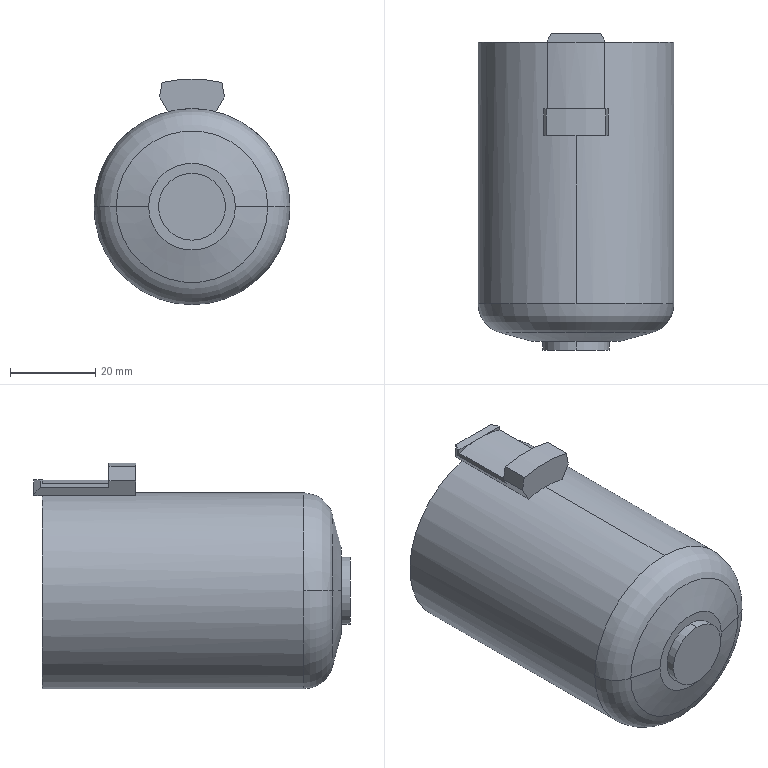Part | STEP file | _AL30-A_BOWL | 1 solid | 29 faces | box 46 x 74.3 x 53 mm | volume 115027 mm3 | plane 17 | cylinder 8 | torus 2 | cone 2 | commonest cylinder face diameters 46 x4 15.7 x2 52 x1 60 x1
STEP:
#1=CARTESIAN_POINT('',(23.,-93.199,0.));
#2=VERTEX_POINT('',#1);
#3=CARTESIAN_POINT('',(0.,-93.199,-23.));
#4=VERTEX_POINT('',#3);
#5=CARTESIAN_POINT('',(0.,-93.199,0.));
#6=DIRECTION('',(0.,1.,0.));
#7=DIRECTION('',(0.,0.,1.));
#8=AXIS2_PLACEMENT_3D('',#5,#6,#7);
#9=CIRCLE('',#8,23.);
#10=EDGE_CURVE('',#2,#4,#9,.T.);
#11=ORIENTED_EDGE('',*,*,#10,.T.);
#12=CARTESIAN_POINT('',(0.,-31.8,-23.));
#13=VERTEX_POINT('',#12);
#14=CARTESIAN_POINT('',(0.,-104.1,-23.));
#15=DIRECTION('',(0.,1.,0.));
#16=VECTOR('',#15,1000.);
#17=LINE('',#14,#16);
#18=EDGE_CURVE('',#4,#13,#17,.T.);
#19=ORIENTED_EDGE('',*,*,#18,.T.);
#20=CARTESIAN_POINT('',(5.604,-31.8,22.307));
#21=VERTEX_POINT('',#20);
#22=CARTESIAN_POINT('',(0.,-31.8,0.));
#23=DIRECTION('',(0.,-1.,0.));
#24=DIRECTION('',(0.,0.,1.));
#25=AXIS2_PLACEMENT_3D('',#22,#23,#24);
#26=CIRCLE('',#25,23.);
#27=EDGE_CURVE('',#13,#21,#26,.T.);
#28=ORIENTED_EDGE('',*,*,#27,.T.);
#29=CARTESIAN_POINT('',(5.604,-53.76,22.307));
#30=VERTEX_POINT('',#29);
#31=CARTESIAN_POINT('',(5.604,-104.1,22.307));
#32=DIRECTION('',(0.,-1.,0.));
#33=VECTOR('',#32,1000.);
#34=LINE('',#31,#33);
#35=EDGE_CURVE('',#21,#30,#34,.T.);
#36=ORIENTED_EDGE('',*,*,#35,.T.);
#37=CARTESIAN_POINT('',(0.,-53.76,23.));
#38=VERTEX_POINT('',#37);
#39=CARTESIAN_POINT('',(0.,-53.76,0.));
#40=DIRECTION('',(0.,-1.,0.));
#41=DIRECTION('',(0.,0.,1.));
#42=AXIS2_PLACEMENT_3D('',#39,#40,#41);
#43=CIRCLE('',#42,23.);
#44=EDGE_CURVE('',#30,#38,#43,.T.);
#45=ORIENTED_EDGE('',*,*,#44,.T.);
#46=CARTESIAN_POINT('',(0.,-93.199,23.));
#47=VERTEX_POINT('',#46);
#48=CARTESIAN_POINT('',(0.,-104.1,23.));
#49=DIRECTION('',(0.,1.,0.));
#50=VECTOR('',#49,1000.);
#51=LINE('',#48,#50);
#52=EDGE_CURVE('',#47,#38,#51,.T.);
#53=ORIENTED_EDGE('',*,*,#52,.F.);
#54=CARTESIAN_POINT('',(0.,-93.199,0.));
#55=DIRECTION('',(0.,1.,0.));
#56=DIRECTION('',(0.,0.,1.));
#57=AXIS2_PLACEMENT_3D('',#54,#55,#56);
#58=CIRCLE('',#57,23.);
#59=EDGE_CURVE('',#47,#2,#58,.T.);
#60=ORIENTED_EDGE('',*,*,#59,.T.);
#61=EDGE_LOOP('',(#11,#19,#28,#36,#45,#53,#60));
#62=FACE_OUTER_BOUND('',#61,.T.);
#63=CARTESIAN_POINT('',(0.,-104.1,0.));
#64=DIRECTION('',(0.,1.,0.));
#65=DIRECTION('',(0.,0.,1.));
#66=AXIS2_PLACEMENT_3D('',#63,#64,#65);
#67=CYLINDRICAL_SURFACE('',#66,23.);
#68=ADVANCED_FACE('',(#62),#67,.T.);
#69=CARTESIAN_POINT('',(-23.,-93.199,0.));
#70=VERTEX_POINT('',#69);
#71=CARTESIAN_POINT('',(0.,-93.199,0.));
#72=DIRECTION('',(0.,1.,0.));
#73=DIRECTION('',(0.,0.,1.));
#74=AXIS2_PLACEMENT_3D('',#71,#72,#73);
#75=CIRCLE('',#74,23.);
#76=EDGE_CURVE('',#70,#47,#75,.T.);
#77=ORIENTED_EDGE('',*,*,#76,.F.);
#78=CARTESIAN_POINT('',(-17.812,-99.96,0.));
#79=VERTEX_POINT('',#78);
#80=CARTESIAN_POINT('',(-16.,-93.199,0.));
#81=DIRECTION('',(0.,0.,1.));
#82=DIRECTION('',(1.,0.,0.));
#83=AXIS2_PLACEMENT_3D('',#80,#81,#82);
#84=CIRCLE('',#83,7.);
#85=EDGE_CURVE('',#70,#79,#84,.T.);
#86=ORIENTED_EDGE('',*,*,#85,.T.);
#87=CARTESIAN_POINT('',(17.812,-99.96,0.));
#88=VERTEX_POINT('',#87);
#89=CARTESIAN_POINT('',(0.,-99.96,0.));
#90=DIRECTION('',(0.,1.,0.));
#91=DIRECTION('',(0.,0.,-1.));
#92=AXIS2_PLACEMENT_3D('',#89,#90,#91);
#93=CIRCLE('',#92,17.812);
#94=EDGE_CURVE('',#79,#88,#93,.T.);
#95=ORIENTED_EDGE('',*,*,#94,.T.);
#96=CARTESIAN_POINT('',(16.,-93.199,0.));
#97=DIRECTION('',(0.,0.,-1.));
#98=DIRECTION('',(-1.,0.,0.));
#99=AXIS2_PLACEMENT_3D('',#96,#97,#98);
#100=CIRCLE('',#99,7.);
#101=EDGE_CURVE('',#2,#88,#100,.T.);
#102=ORIENTED_EDGE('',*,*,#101,.F.);
#103=ORIENTED_EDGE('',*,*,#59,.F.);
#104=EDGE_LOOP('',(#77,#86,#95,#102,#103));
#105=FACE_OUTER_BOUND('',#104,.T.);
#106=CARTESIAN_POINT('',(0.,-93.199,0.));
#107=DIRECTION('',(0.,-1.,0.));
#108=DIRECTION('',(1.,0.,0.));
#109=AXIS2_PLACEMENT_3D('',#106,#107,#108);
#110=TOROIDAL_SURFACE('',#109,16.,7.);
#111=ADVANCED_FACE('',(#105),#110,.T.);
#112=CARTESIAN_POINT('',(0.,-31.8,23.));
#113=VERTEX_POINT('',#112);
#114=CARTESIAN_POINT('',(0.,-31.8,0.));
#115=DIRECTION('',(0.,-1.,0.));
#116=DIRECTION('',(0.,0.,1.));
#117=AXIS2_PLACEMENT_3D('',#114,#115,#116);
#118=CIRCLE('',#117,23.);
#119=EDGE_CURVE('',#21,#113,#118,.T.);
#120=ORIENTED_EDGE('',*,*,#119,.T.);
#121=CARTESIAN_POINT('',(0.,-29.8,23.));
#122=VERTEX_POINT('',#121);
#123=CARTESIAN_POINT('',(0.,-29.8,23.));
#124=DIRECTION('',(0.,1.,0.));
#125=VECTOR('',#124,1000.);
#126=LINE('',#123,#125);
#127=EDGE_CURVE('',#113,#122,#126,.T.);
#128=ORIENTED_EDGE('',*,*,#127,.T.);
#129=CARTESIAN_POINT('',(5.604,-29.8,22.307));
#130=VERTEX_POINT('',#129);
#131=CARTESIAN_POINT('',(0.,-29.8,0.));
#132=DIRECTION('',(0.,-1.,0.));
#133=DIRECTION('',(0.,0.,1.));
#134=AXIS2_PLACEMENT_3D('',#131,#132,#133);
#135=CIRCLE('',#134,23.);
#136=EDGE_CURVE('',#130,#122,#135,.T.);
#137=ORIENTED_EDGE('',*,*,#136,.F.);
#138=CARTESIAN_POINT('',(5.604,-47.45,22.307));
#139=DIRECTION('',(0.,1.,0.));
#140=VECTOR('',#139,1000.);
#141=LINE('',#138,#140);
#142=EDGE_CURVE('',#21,#130,#141,.T.);
#143=ORIENTED_EDGE('',*,*,#142,.F.);
#144=EDGE_LOOP('',(#120,#128,#137,#143));
#145=FACE_OUTER_BOUND('',#144,.T.);
#146=CARTESIAN_POINT('',(0.,-29.8,0.));
#147=DIRECTION('',(0.,1.,0.));
#148=DIRECTION('',(0.,0.,1.));
#149=AXIS2_PLACEMENT_3D('',#146,#147,#148);
#150=CYLINDRICAL_SURFACE('',#149,23.);
#151=ADVANCED_FACE('',(#145),#150,.F.);
#152=CARTESIAN_POINT('',(-10.2,-102.,0.));
#153=VERTEX_POINT('',#152);
#154=CARTESIAN_POINT('',(10.2,-102.,0.));
#155=VERTEX_POINT('',#154);
#156=CARTESIAN_POINT('',(0.,-102.,0.));
#157=DIRECTION('',(0.,1.,0.));
#158=DIRECTION('',(-1.,0.,0.));
#159=AXIS2_PLACEMENT_3D('',#156,#157,#158);
#160=CIRCLE('',#159,10.2);
#161=EDGE_CURVE('',#153,#155,#160,.T.);
#162=ORIENTED_EDGE('',*,*,#161,.T.);
#163=CARTESIAN_POINT('',(17.812,-99.96,0.));
#164=DIRECTION('',(0.9659,0.2588,0.));
#165=VECTOR('',#164,1000.);
#166=LINE('',#163,#165);
#167=EDGE_CURVE('',#155,#88,#166,.T.);
#168=ORIENTED_EDGE('',*,*,#167,.T.);
#169=ORIENTED_EDGE('',*,*,#94,.F.);
#170=CARTESIAN_POINT('',(-17.812,-99.96,0.));
#171=DIRECTION('',(-0.9659,0.2588,0.));
#172=VECTOR('',#171,1000.);
#173=LINE('',#170,#172);
#174=EDGE_CURVE('',#153,#79,#173,.T.);
#175=ORIENTED_EDGE('',*,*,#174,.F.);
#176=EDGE_LOOP('',(#162,#168,#169,#175));
#177=FACE_OUTER_BOUND('',#176,.T.);
#178=CARTESIAN_POINT('',(0.,-99.96,0.));
#179=DIRECTION('',(0.,1.,0.));
#180=DIRECTION('',(-1.,0.,0.));
#181=AXIS2_PLACEMENT_3D('',#178,#179,#180);
#182=CONICAL_SURFACE('',#181,17.812,1.309);
#183=ADVANCED_FACE('',(#177),#182,.T.);
#184=CARTESIAN_POINT('',(0.,-104.1,7.85));
#185=VERTEX_POINT('',#184);
#186=CARTESIAN_POINT('',(0.,-104.1,-7.85));
#187=VERTEX_POINT('',#186);
#188=CARTESIAN_POINT('',(0.,-104.1,0.));
#189=DIRECTION('',(0.,1.,0.));
#190=DIRECTION('',(0.,0.,1.));
#191=AXIS2_PLACEMENT_3D('',#188,#189,#190);
#192=CIRCLE('',#191,7.85);
#193=EDGE_CURVE('',#185,#187,#192,.T.);
#194=ORIENTED_EDGE('',*,*,#193,.T.);
#195=CARTESIAN_POINT('',(0.,-102.,-7.85));
#196=VERTEX_POINT('',#195);
#197=CARTESIAN_POINT('',(0.,-104.1,-7.85));
#198=DIRECTION('',(0.,1.,0.));
#199=VECTOR('',#198,1000.);
#200=LINE('',#197,#199);
#201=EDGE_CURVE('',#187,#196,#200,.T.);
#202=ORIENTED_EDGE('',*,*,#201,.T.);
#203=CARTESIAN_POINT('',(0.,-102.,7.85));
#204=VERTEX_POINT('',#203);
#205=CARTESIAN_POINT('',(0.,-102.,0.));
#206=DIRECTION('',(0.,-1.,0.));
#207=DIRECTION('',(0.,0.,1.));
#208=AXIS2_PLACEMENT_3D('',#205,#206,#207);
#209=CIRCLE('',#208,7.85);
#210=EDGE_CURVE('',#196,#204,#209,.T.);
#211=ORIENTED_EDGE('',*,*,#210,.T.);
#212=CARTESIAN_POINT('',(0.,-104.1,7.85));
#213=DIRECTION('',(0.,1.,0.));
#214=VECTOR('',#213,1000.);
#215=LINE('',#212,#214);
#216=EDGE_CURVE('',#185,#204,#215,.T.);
#217=ORIENTED_EDGE('',*,*,#216,.F.);
#218=EDGE_LOOP('',(#194,#202,#211,#217));
#219=FACE_OUTER_BOUND('',#218,.T.);
#220=CARTESIAN_POINT('',(0.,-104.1,0.));
#221=DIRECTION('',(0.,1.,0.));
#222=DIRECTION('',(0.,0.,1.));
#223=AXIS2_PLACEMENT_3D('',#220,#221,#222);
#224=CYLINDRICAL_SURFACE('',#223,7.85);
#225=ADVANCED_FACE('',(#219),#224,.T.);
#226=ORIENTED_EDGE('',*,*,#18,.F.);
#227=CARTESIAN_POINT('',(0.,-93.199,0.));
#228=DIRECTION('',(0.,1.,0.));
#229=DIRECTION('',(0.,0.,1.));
#230=AXIS2_PLACEMENT_3D('',#227,#228,#229);
#231=CIRCLE('',#230,23.);
#232=EDGE_CURVE('',#4,#70,#231,.T.);
#233=ORIENTED_EDGE('',*,*,#232,.T.);
#234=ORIENTED_EDGE('',*,*,#76,.T.);
#235=ORIENTED_EDGE('',*,*,#52,.T.);
#236=CARTESIAN_POINT('',(-5.604,-53.76,22.307));
#237=VERTEX_POINT('',#236);
#238=CARTESIAN_POINT('',(0.,-53.76,0.));
#239=DIRECTION('',(0.,-1.,0.));
#240=DIRECTION('',(0.,0.,1.));
#241=AXIS2_PLACEMENT_3D('',#238,#239,#240);
#242=CIRCLE('',#241,23.);
#243=EDGE_CURVE('',#38,#237,#242,.T.);
#244=ORIENTED_EDGE('',*,*,#243,.T.);
#245=CARTESIAN_POINT('',(-5.604,-31.8,22.307));
#246=VERTEX_POINT('',#245);
#247=CARTESIAN_POINT('',(-5.604,-104.1,22.307));
#248=DIRECTION('',(0.,1.,0.));
#249=VECTOR('',#248,1000.);
#250=LINE('',#247,#249);
#251=EDGE_CURVE('',#237,#246,#250,.T.);
#252=ORIENTED_EDGE('',*,*,#251,.T.);
#253=CARTESIAN_POINT('',(0.,-31.8,0.));
#254=DIRECTION('',(0.,-1.,0.));
#255=DIRECTION('',(0.,0.,1.));
#256=AXIS2_PLACEMENT_3D('',#253,#254,#255);
#257=CIRCLE('',#256,23.);
#258=EDGE_CURVE('',#246,#13,#257,.T.);
#259=ORIENTED_EDGE('',*,*,#258,.T.);
#260=EDGE_LOOP('',(#226,#233,#234,#235,#244,#252,#259));
#261=FACE_OUTER_BOUND('',#260,.T.);
#262=CARTESIAN_POINT('',(0.,-104.1,0.));
#263=DIRECTION('',(0.,1.,0.));
#264=DIRECTION('',(0.,0.,1.));
#265=AXIS2_PLACEMENT_3D('',#262,#263,#264);
#266=CYLINDRICAL_SURFACE('',#265,23.);
#267=ADVANCED_FACE('',(#261),#266,.T.);
#268=CARTESIAN_POINT('',(7.6,-53.76,25.765));
#269=VERTEX_POINT('',#268);
#270=CARTESIAN_POINT('',(7.6,-53.76,25.765));
#271=DIRECTION('',(-0.5,0.,-0.866));
#272=VECTOR('',#271,1000.);
#273=LINE('',#270,#272);
#274=EDGE_CURVE('',#269,#30,#273,.T.);
#275=ORIENTED_EDGE('',*,*,#274,.F.);
#276=CARTESIAN_POINT('',(7.004,-53.76,29.171));
#277=VERTEX_POINT('',#276);
#278=CARTESIAN_POINT('',(7.004,-53.76,29.171));
#279=DIRECTION('',(0.1723,0.,-0.985));
#280=VECTOR('',#279,1000.);
#281=LINE('',#278,#280);
#282=EDGE_CURVE('',#277,#269,#281,.T.);
#283=ORIENTED_EDGE('',*,*,#282,.F.);
#284=CARTESIAN_POINT('',(-7.004,-53.76,29.171));
#285=VERTEX_POINT('',#284);
#286=CARTESIAN_POINT('',(0.,-53.76,0.));
#287=DIRECTION('',(0.,1.,0.));
#288=DIRECTION('',(0.,0.,-1.));
#289=AXIS2_PLACEMENT_3D('',#286,#287,#288);
#290=CIRCLE('',#289,30.);
#291=EDGE_CURVE('',#285,#277,#290,.T.);
#292=ORIENTED_EDGE('',*,*,#291,.F.);
#293=CARTESIAN_POINT('',(-7.6,-53.76,25.765));
#294=VERTEX_POINT('',#293);
#295=CARTESIAN_POINT('',(-7.6,-53.76,25.765));
#296=DIRECTION('',(0.1723,0.,0.985));
#297=VECTOR('',#296,1000.);
#298=LINE('',#295,#297);
#299=EDGE_CURVE('',#294,#285,#298,.T.);
#300=ORIENTED_EDGE('',*,*,#299,.F.);
#301=CARTESIAN_POINT('',(-5.604,-53.76,22.307));
#302=DIRECTION('',(-0.5,0.,0.866));
#303=VECTOR('',#302,1000.);
#304=LINE('',#301,#303);
#305=EDGE_CURVE('',#237,#294,#304,.T.);
#306=ORIENTED_EDGE('',*,*,#305,.F.);
#307=ORIENTED_EDGE('',*,*,#243,.F.);
#308=ORIENTED_EDGE('',*,*,#44,.F.);
#309=EDGE_LOOP('',(#275,#283,#292,#300,#306,#307,#308));
#310=FACE_OUTER_BOUND('',#309,.T.);
#311=CARTESIAN_POINT('',(0.,-53.76,0.));
#312=DIRECTION('',(0.,1.,0.));
#313=DIRECTION('',(0.,0.,1.));
#314=AXIS2_PLACEMENT_3D('',#311,#312,#313);
#315=PLANE('',#314);
#316=ADVANCED_FACE('',(#310),#315,.F.);
#317=CARTESIAN_POINT('',(7.6,-47.45,25.765));
#318=VERTEX_POINT('',#317);
#319=CARTESIAN_POINT('',(7.6,-47.45,25.765));
#320=DIRECTION('',(0.,-1.,0.));
#321=VECTOR('',#320,1000.);
#322=LINE('',#319,#321);
#323=EDGE_CURVE('',#318,#269,#322,.T.);
#324=ORIENTED_EDGE('',*,*,#323,.T.);
#325=ORIENTED_EDGE('',*,*,#274,.T.);
#326=ORIENTED_EDGE('',*,*,#35,.F.);
#327=ORIENTED_EDGE('',*,*,#142,.T.);
#328=CARTESIAN_POINT('',(5.798,-29.8,22.644));
#329=VERTEX_POINT('',#328);
#330=CARTESIAN_POINT('',(5.798,-29.8,22.644));
#331=DIRECTION('',(-0.5,0.,-0.866));
#332=VECTOR('',#331,1000.);
#333=LINE('',#330,#332);
#334=EDGE_CURVE('',#329,#130,#333,.T.);
#335=ORIENTED_EDGE('',*,*,#334,.F.);
#336=CARTESIAN_POINT('',(6.7,-31.301,24.206));
#337=VERTEX_POINT('',#336);
#338=CARTESIAN_POINT('',(5.798,-29.8,22.644));
#339=DIRECTION('',(0.3843,-0.6396,0.6657));
#340=VECTOR('',#339,1000.);
#341=LINE('',#338,#340);
#342=EDGE_CURVE('',#329,#337,#341,.T.);
#343=ORIENTED_EDGE('',*,*,#342,.T.);
#344=CARTESIAN_POINT('',(6.7,-47.45,24.206));
#345=VERTEX_POINT('',#344);
#346=CARTESIAN_POINT('',(6.7,-47.45,24.206));
#347=DIRECTION('',(0.,-1.,0.));
#348=VECTOR('',#347,1000.);
#349=LINE('',#346,#348);
#350=EDGE_CURVE('',#337,#345,#349,.T.);
#351=ORIENTED_EDGE('',*,*,#350,.T.);
#352=CARTESIAN_POINT('',(6.7,-47.45,24.206));
#353=DIRECTION('',(0.5,0.,0.866));
#354=VECTOR('',#353,1000.);
#355=LINE('',#352,#354);
#356=EDGE_CURVE('',#345,#318,#355,.T.);
#357=ORIENTED_EDGE('',*,*,#356,.T.);
#358=EDGE_LOOP('',(#324,#325,#326,#327,#335,#343,#351,#357));
#359=FACE_OUTER_BOUND('',#358,.T.);
#360=CARTESIAN_POINT('',(6.7,-47.45,24.206));
#361=DIRECTION('',(0.866,0.,-0.5));
#362=DIRECTION('',(-0.5,0.,-0.866));
#363=AXIS2_PLACEMENT_3D('',#360,#361,#362);
#364=PLANE('',#363);
#365=ADVANCED_FACE('',(#359),#364,.T.);
#366=ORIENTED_EDGE('',*,*,#258,.F.);
#367=CARTESIAN_POINT('',(0.,-31.8,0.));
#368=DIRECTION('',(0.,-1.,0.));
#369=DIRECTION('',(0.,0.,1.));
#370=AXIS2_PLACEMENT_3D('',#367,#368,#369);
#371=CIRCLE('',#370,23.);
#372=EDGE_CURVE('',#113,#246,#371,.T.);
#373=ORIENTED_EDGE('',*,*,#372,.F.);
#374=ORIENTED_EDGE('',*,*,#119,.F.);
#375=ORIENTED_EDGE('',*,*,#27,.F.);
#376=EDGE_LOOP('',(#366,#373,#374,#375));
#377=FACE_OUTER_BOUND('',#376,.T.);
#378=CARTESIAN_POINT('',(0.,-31.8,0.));
#379=DIRECTION('',(0.,-1.,0.));
#380=DIRECTION('',(0.,0.,-1.));
#381=AXIS2_PLACEMENT_3D('',#378,#379,#380);
#382=PLANE('',#381);
#383=ADVANCED_FACE('',(#377),#382,.F.);
#384=ORIENTED_EDGE('',*,*,#85,.F.);
#385=ORIENTED_EDGE('',*,*,#232,.F.);
#386=ORIENTED_EDGE('',*,*,#10,.F.);
#387=ORIENTED_EDGE('',*,*,#101,.T.);
#388=CARTESIAN_POINT('',(0.,-99.96,0.));
#389=DIRECTION('',(0.,1.,0.));
#390=DIRECTION('',(0.,0.,-1.));
#391=AXIS2_PLACEMENT_3D('',#388,#389,#390);
#392=CIRCLE('',#391,17.812);
#393=EDGE_CURVE('',#88,#79,#392,.T.);
#394=ORIENTED_EDGE('',*,*,#393,.T.);
#395=EDGE_LOOP('',(#384,#385,#386,#387,#394));
#396=FACE_OUTER_BOUND('',#395,.T.);
#397=CARTESIAN_POINT('',(0.,-93.199,0.));
#398=DIRECTION('',(0.,-1.,0.));
#399=DIRECTION('',(1.,0.,0.));
#400=AXIS2_PLACEMENT_3D('',#397,#398,#399);
#401=TOROIDAL_SURFACE('',#400,16.,7.);
#402=ADVANCED_FACE('',(#396),#401,.T.);
#403=ORIENTED_EDGE('',*,*,#251,.F.);
#404=ORIENTED_EDGE('',*,*,#305,.T.);
#405=CARTESIAN_POINT('',(-7.6,-47.45,25.765));
#406=VERTEX_POINT('',#405);
#407=CARTESIAN_POINT('',(-7.6,-47.45,25.765));
#408=DIRECTION('',(0.,1.,0.));
#409=VECTOR('',#408,1000.);
#410=LINE('',#407,#409);
#411=EDGE_CURVE('',#294,#406,#410,.T.);
#412=ORIENTED_EDGE('',*,*,#411,.T.);
#413=CARTESIAN_POINT('',(-6.7,-47.45,24.206));
#414=VERTEX_POINT('',#413);
#415=CARTESIAN_POINT('',(-5.541,-47.45,22.199));
#416=DIRECTION('',(0.5,0.,-0.866));
#417=VECTOR('',#416,1000.);
#418=LINE('',#415,#417);
#419=EDGE_CURVE('',#406,#414,#418,.T.);
#420=ORIENTED_EDGE('',*,*,#419,.T.);
#421=CARTESIAN_POINT('',(-6.7,-31.301,24.206));
#422=VERTEX_POINT('',#421);
#423=CARTESIAN_POINT('',(-6.7,-47.45,24.206));
#424=DIRECTION('',(0.,1.,0.));
#425=VECTOR('',#424,1000.);
#426=LINE('',#423,#425);
#427=EDGE_CURVE('',#414,#422,#426,.T.);
#428=ORIENTED_EDGE('',*,*,#427,.T.);
#429=CARTESIAN_POINT('',(-5.798,-29.8,22.644));
#430=VERTEX_POINT('',#429);
#431=CARTESIAN_POINT('',(-6.7,-31.301,24.206));
#432=DIRECTION('',(0.3843,0.6396,-0.6657));
#433=VECTOR('',#432,1000.);
#434=LINE('',#431,#433);
#435=EDGE_CURVE('',#422,#430,#434,.T.);
#436=ORIENTED_EDGE('',*,*,#435,.T.);
#437=CARTESIAN_POINT('',(-5.604,-29.8,22.307));
#438=VERTEX_POINT('',#437);
#439=CARTESIAN_POINT('',(-5.604,-29.8,22.307));
#440=DIRECTION('',(-0.5,0.,0.866));
#441=VECTOR('',#440,1000.);
#442=LINE('',#439,#441);
#443=EDGE_CURVE('',#438,#430,#442,.T.);
#444=ORIENTED_EDGE('',*,*,#443,.F.);
#445=CARTESIAN_POINT('',(-5.604,-47.45,22.307));
#446=DIRECTION('',(0.,-1.,0.));
#447=VECTOR('',#446,1000.);
#448=LINE('',#445,#447);
#449=EDGE_CURVE('',#438,#246,#448,.T.);
#450=ORIENTED_EDGE('',*,*,#449,.T.);
#451=EDGE_LOOP('',(#403,#404,#412,#420,#428,#436,#444,#450));
#452=FACE_OUTER_BOUND('',#451,.T.);
#453=CARTESIAN_POINT('',(-5.541,-47.45,22.199));
#454=DIRECTION('',(-0.866,0.,-0.5));
#455=DIRECTION('',(-0.5,0.,0.866));
#456=AXIS2_PLACEMENT_3D('',#453,#454,#455);
#457=PLANE('',#456);
#458=ADVANCED_FACE('',(#452),#457,.T.);
#459=CARTESIAN_POINT('',(7.004,-47.45,29.171));
#460=VERTEX_POINT('',#459);
#461=CARTESIAN_POINT('',(7.004,-47.45,29.171));
#462=DIRECTION('',(-0.1723,0.,0.985));
#463=VECTOR('',#462,1000.);
#464=LINE('',#461,#463);
#465=EDGE_CURVE('',#318,#460,#464,.T.);
#466=ORIENTED_EDGE('',*,*,#465,.T.);
#467=CARTESIAN_POINT('',(7.004,-53.76,29.171));
#468=DIRECTION('',(0.,-1.,0.));
#469=VECTOR('',#468,1000.);
#470=LINE('',#467,#469);
#471=EDGE_CURVE('',#460,#277,#470,.T.);
#472=ORIENTED_EDGE('',*,*,#471,.T.);
#473=ORIENTED_EDGE('',*,*,#282,.T.);
#474=ORIENTED_EDGE('',*,*,#323,.F.);
#475=EDGE_LOOP('',(#466,#472,#473,#474));
#476=FACE_OUTER_BOUND('',#475,.T.);
#477=CARTESIAN_POINT('',(7.004,-53.76,29.171));
#478=DIRECTION('',(0.985,0.,0.1723));
#479=DIRECTION('',(0.1723,0.,-0.985));
#480=AXIS2_PLACEMENT_3D('',#477,#478,#479);
#481=PLANE('',#480);
#482=ADVANCED_FACE('',(#476),#481,.T.);
#483=CARTESIAN_POINT('',(-7.004,-47.45,29.171));
#484=VERTEX_POINT('',#483);
#485=CARTESIAN_POINT('',(0.,-47.45,0.));
#486=DIRECTION('',(0.,-1.,0.));
#487=DIRECTION('',(0.,0.,-1.));
#488=AXIS2_PLACEMENT_3D('',#485,#486,#487);
#489=CIRCLE('',#488,30.);
#490=EDGE_CURVE('',#460,#484,#489,.T.);
#491=ORIENTED_EDGE('',*,*,#490,.T.);
#492=CARTESIAN_POINT('',(-7.004,-53.76,29.171));
#493=DIRECTION('',(0.,-1.,0.));
#494=VECTOR('',#493,1000.);
#495=LINE('',#492,#494);
#496=EDGE_CURVE('',#484,#285,#495,.T.);
#497=ORIENTED_EDGE('',*,*,#496,.T.);
#498=ORIENTED_EDGE('',*,*,#291,.T.);
#499=ORIENTED_EDGE('',*,*,#471,.F.);
#500=EDGE_LOOP('',(#491,#497,#498,#499));
#501=FACE_OUTER_BOUND('',#500,.T.);
#502=CARTESIAN_POINT('',(0.,-53.76,0.));
#503=DIRECTION('',(0.,-1.,0.));
#504=DIRECTION('',(0.,0.,-1.));
#505=AXIS2_PLACEMENT_3D('',#502,#503,#504);
#506=CYLINDRICAL_SURFACE('',#505,30.);
#507=ADVANCED_FACE('',(#501),#506,.T.);
#508=CARTESIAN_POINT('',(-7.6,-47.45,25.765));
#509=DIRECTION('',(-0.1723,0.,-0.985));
#510=VECTOR('',#509,1000.);
#511=LINE('',#508,#510);
#512=EDGE_CURVE('',#484,#406,#511,.T.);
#513=ORIENTED_EDGE('',*,*,#512,.T.);
#514=ORIENTED_EDGE('',*,*,#411,.F.);
#515=ORIENTED_EDGE('',*,*,#299,.T.);
#516=ORIENTED_EDGE('',*,*,#496,.F.);
#517=EDGE_LOOP('',(#513,#514,#515,#516));
#518=FACE_OUTER_BOUND('',#517,.T.);
#519=CARTESIAN_POINT('',(-7.6,-53.76,25.765));
#520=DIRECTION('',(-0.985,0.,0.1723));
#521=DIRECTION('',(0.1723,0.,0.985));
#522=AXIS2_PLACEMENT_3D('',#519,#520,#521);
#523=PLANE('',#522);
#524=ADVANCED_FACE('',(#518),#523,.T.);
#525=ORIENTED_EDGE('',*,*,#490,.F.);
#526=ORIENTED_EDGE('',*,*,#465,.F.);
#527=ORIENTED_EDGE('',*,*,#356,.F.);
#528=CARTESIAN_POINT('',(6.7,-47.45,25.122));
#529=VERTEX_POINT('',#528);
#530=CARTESIAN_POINT('',(6.7,-47.45,0.));
#531=DIRECTION('',(0.,0.,1.));
#532=VECTOR('',#531,1000.);
#533=LINE('',#530,#532);
#534=EDGE_CURVE('',#345,#529,#533,.T.);
#535=ORIENTED_EDGE('',*,*,#534,.T.);
#536=CARTESIAN_POINT('',(-6.7,-47.45,25.122));
#537=VERTEX_POINT('',#536);
#538=CARTESIAN_POINT('',(0.,-47.45,0.));
#539=DIRECTION('',(0.,-1.,0.));
#540=DIRECTION('',(0.,0.,-1.));
#541=AXIS2_PLACEMENT_3D('',#538,#539,#540);
#542=CIRCLE('',#541,26.);
#543=EDGE_CURVE('',#529,#537,#542,.T.);
#544=ORIENTED_EDGE('',*,*,#543,.T.);
#545=CARTESIAN_POINT('',(-6.7,-47.45,0.));
#546=DIRECTION('',(0.,0.,-1.));
#547=VECTOR('',#546,1000.);
#548=LINE('',#545,#547);
#549=EDGE_CURVE('',#537,#414,#548,.T.);
#550=ORIENTED_EDGE('',*,*,#549,.T.);
#551=ORIENTED_EDGE('',*,*,#419,.F.);
#552=ORIENTED_EDGE('',*,*,#512,.F.);
#553=EDGE_LOOP('',(#525,#526,#527,#535,#544,#550,#551,#552));
#554=FACE_OUTER_BOUND('',#553,.T.);
#555=CARTESIAN_POINT('',(0.,-47.45,0.));
#556=DIRECTION('',(0.,1.,0.));
#557=DIRECTION('',(0.,0.,1.));
#558=AXIS2_PLACEMENT_3D('',#555,#556,#557);
#559=PLANE('',#558);
#560=ADVANCED_FACE('',(#554),#559,.T.);
#561=CARTESIAN_POINT('',(6.7,-31.301,26.));
#562=VERTEX_POINT('',#561);
#563=CARTESIAN_POINT('',(6.7,-31.8,26.));
#564=VERTEX_POINT('',#563);
#565=CARTESIAN_POINT('',(6.7,-29.8,26.));
#566=DIRECTION('',(0.,-1.,0.));
#567=VECTOR('',#566,1000.);
#568=LINE('',#565,#567);
#569=EDGE_CURVE('',#562,#564,#568,.T.);
#570=ORIENTED_EDGE('',*,*,#569,.T.);
#571=CARTESIAN_POINT('',(6.7,-31.8,25.122));
#572=VERTEX_POINT('',#571);
#573=CARTESIAN_POINT('',(6.7,-31.8,0.));
#574=DIRECTION('',(0.,0.,-1.));
#575=VECTOR('',#574,1000.);
#576=LINE('',#573,#575);
#577=EDGE_CURVE('',#564,#572,#576,.T.);
#578=ORIENTED_EDGE('',*,*,#577,.T.);
#579=CARTESIAN_POINT('',(6.7,-47.45,25.122));
#580=DIRECTION('',(0.,-1.,0.));
#581=VECTOR('',#580,1000.);
#582=LINE('',#579,#581);
#583=EDGE_CURVE('',#572,#529,#582,.T.);
#584=ORIENTED_EDGE('',*,*,#583,.T.);
#585=ORIENTED_EDGE('',*,*,#534,.F.);
#586=ORIENTED_EDGE('',*,*,#350,.F.);
#587=CARTESIAN_POINT('',(6.7,-31.301,25.122));
#588=DIRECTION('',(0.,0.,1.));
#589=VECTOR('',#588,1000.);
#590=LINE('',#587,#589);
#591=EDGE_CURVE('',#337,#562,#590,.T.);
#592=ORIENTED_EDGE('',*,*,#591,.T.);
#593=EDGE_LOOP('',(#570,#578,#584,#585,#586,#592));
#594=FACE_OUTER_BOUND('',#593,.T.);
#595=CARTESIAN_POINT('',(6.7,-47.45,25.122));
#596=DIRECTION('',(1.,0.,0.));
#597=DIRECTION('',(0.,0.,-1.));
#598=AXIS2_PLACEMENT_3D('',#595,#596,#597);
#599=PLANE('',#598);
#600=ADVANCED_FACE('',(#594),#599,.T.);
#601=CARTESIAN_POINT('',(5.798,-29.8,26.));
#602=VERTEX_POINT('',#601);
#603=CARTESIAN_POINT('',(5.798,-29.8,28.));
#604=DIRECTION('',(0.,0.,1.));
#605=VECTOR('',#604,1000.);
#606=LINE('',#603,#605);
#607=EDGE_CURVE('',#329,#602,#606,.T.);
#608=ORIENTED_EDGE('',*,*,#607,.T.);
#609=CARTESIAN_POINT('',(5.798,-29.8,26.));
#610=DIRECTION('',(0.515,-0.8572,0.));
#611=VECTOR('',#610,1000.);
#612=LINE('',#609,#611);
#613=EDGE_CURVE('',#602,#562,#612,.T.);
#614=ORIENTED_EDGE('',*,*,#613,.T.);
#615=ORIENTED_EDGE('',*,*,#591,.F.);
#616=ORIENTED_EDGE('',*,*,#342,.F.);
#617=EDGE_LOOP('',(#608,#614,#615,#616));
#618=FACE_OUTER_BOUND('',#617,.T.);
#619=CARTESIAN_POINT('',(5.798,-29.8,28.));
#620=DIRECTION('',(0.8572,0.515,0.));
#621=DIRECTION('',(-0.515,0.8572,0.));
#622=AXIS2_PLACEMENT_3D('',#619,#620,#621);
#623=PLANE('',#622);
#624=ADVANCED_FACE('',(#618),#623,.T.);
#625=ORIENTED_EDGE('',*,*,#127,.F.);
#626=ORIENTED_EDGE('',*,*,#372,.T.);
#627=ORIENTED_EDGE('',*,*,#449,.F.);
#628=CARTESIAN_POINT('',(0.,-29.8,0.));
#629=DIRECTION('',(0.,-1.,0.));
#630=DIRECTION('',(0.,0.,1.));
#631=AXIS2_PLACEMENT_3D('',#628,#629,#630);
#632=CIRCLE('',#631,23.);
#633=EDGE_CURVE('',#122,#438,#632,.T.);
#634=ORIENTED_EDGE('',*,*,#633,.F.);
#635=EDGE_LOOP('',(#625,#626,#627,#634));
#636=FACE_OUTER_BOUND('',#635,.T.);
#637=CARTESIAN_POINT('',(0.,-29.8,0.));
#638=DIRECTION('',(0.,1.,0.));
#639=DIRECTION('',(0.,0.,1.));
#640=AXIS2_PLACEMENT_3D('',#637,#638,#639);
#641=CYLINDRICAL_SURFACE('',#640,23.);
#642=ADVANCED_FACE('',(#636),#641,.F.);
#643=ORIENTED_EDGE('',*,*,#167,.F.);
#644=CARTESIAN_POINT('',(0.,-102.,0.));
#645=DIRECTION('',(0.,1.,0.));
#646=DIRECTION('',(-1.,0.,0.));
#647=AXIS2_PLACEMENT_3D('',#644,#645,#646);
#648=CIRCLE('',#647,10.2);
#649=EDGE_CURVE('',#155,#153,#648,.T.);
#650=ORIENTED_EDGE('',*,*,#649,.T.);
#651=ORIENTED_EDGE('',*,*,#174,.T.);
#652=ORIENTED_EDGE('',*,*,#393,.F.);
#653=EDGE_LOOP('',(#643,#650,#651,#652));
#654=FACE_OUTER_BOUND('',#653,.T.);
#655=CARTESIAN_POINT('',(0.,-99.96,0.));
#656=DIRECTION('',(0.,1.,0.));
#657=DIRECTION('',(-1.,0.,0.));
#658=AXIS2_PLACEMENT_3D('',#655,#656,#657);
#659=CONICAL_SURFACE('',#658,17.812,1.309);
#660=ADVANCED_FACE('',(#654),#659,.T.);
#661=CARTESIAN_POINT('',(-6.7,-31.301,26.));
#662=VERTEX_POINT('',#661);
#663=CARTESIAN_POINT('',(-6.7,-31.301,28.));
#664=DIRECTION('',(0.,0.,1.));
#665=VECTOR('',#664,1000.);
#666=LINE('',#663,#665);
#667=EDGE_CURVE('',#422,#662,#666,.T.);
#668=ORIENTED_EDGE('',*,*,#667,.T.);
#669=CARTESIAN_POINT('',(-5.798,-29.8,26.));
#670=VERTEX_POINT('',#669);
#671=CARTESIAN_POINT('',(-7.,-31.8,26.));
#672=DIRECTION('',(0.515,0.8572,0.));
#673=VECTOR('',#672,1000.);
#674=LINE('',#671,#673);
#675=EDGE_CURVE('',#662,#670,#674,.T.);
#676=ORIENTED_EDGE('',*,*,#675,.T.);
#677=CARTESIAN_POINT('',(-5.798,-29.8,28.));
#678=DIRECTION('',(0.,0.,-1.));
#679=VECTOR('',#678,1000.);
#680=LINE('',#677,#679);
#681=EDGE_CURVE('',#670,#430,#680,.T.);
#682=ORIENTED_EDGE('',*,*,#681,.T.);
#683=ORIENTED_EDGE('',*,*,#435,.F.);
#684=EDGE_LOOP('',(#668,#676,#682,#683));
#685=FACE_OUTER_BOUND('',#684,.T.);
#686=CARTESIAN_POINT('',(-7.,-31.8,28.));
#687=DIRECTION('',(-0.8572,0.515,0.));
#688=DIRECTION('',(-0.515,-0.8572,0.));
#689=AXIS2_PLACEMENT_3D('',#686,#687,#688);
#690=PLANE('',#689);
#691=ADVANCED_FACE('',(#685),#690,.T.);
#692=ORIENTED_EDGE('',*,*,#427,.F.);
#693=ORIENTED_EDGE('',*,*,#549,.F.);
#694=CARTESIAN_POINT('',(-6.7,-31.8,25.122));
#695=VERTEX_POINT('',#694);
#696=CARTESIAN_POINT('',(-6.7,-47.45,25.122));
#697=DIRECTION('',(0.,1.,0.));
#698=VECTOR('',#697,1000.);
#699=LINE('',#696,#698);
#700=EDGE_CURVE('',#537,#695,#699,.T.);
#701=ORIENTED_EDGE('',*,*,#700,.T.);
#702=CARTESIAN_POINT('',(-6.7,-31.8,26.));
#703=VERTEX_POINT('',#702);
#704=CARTESIAN_POINT('',(-6.7,-31.8,0.));
#705=DIRECTION('',(0.,0.,1.));
#706=VECTOR('',#705,1000.);
#707=LINE('',#704,#706);
#708=EDGE_CURVE('',#695,#703,#707,.T.);
#709=ORIENTED_EDGE('',*,*,#708,.T.);
#710=CARTESIAN_POINT('',(-6.7,-47.45,26.));
#711=DIRECTION('',(0.,1.,0.));
#712=VECTOR('',#711,1000.);
#713=LINE('',#710,#712);
#714=EDGE_CURVE('',#703,#662,#713,.T.);
#715=ORIENTED_EDGE('',*,*,#714,.T.);
#716=ORIENTED_EDGE('',*,*,#667,.F.);
#717=EDGE_LOOP('',(#692,#693,#701,#709,#715,#716));
#718=FACE_OUTER_BOUND('',#717,.T.);
#719=CARTESIAN_POINT('',(-6.7,-47.45,24.206));
#720=DIRECTION('',(-1.,0.,0.));
#721=DIRECTION('',(0.,0.,1.));
#722=AXIS2_PLACEMENT_3D('',#719,#720,#721);
#723=PLANE('',#722);
#724=ADVANCED_FACE('',(#718),#723,.T.);
#725=ORIENTED_EDGE('',*,*,#700,.F.);
#726=ORIENTED_EDGE('',*,*,#543,.F.);
#727=ORIENTED_EDGE('',*,*,#583,.F.);
#728=CARTESIAN_POINT('',(0.,-31.8,26.));
#729=VERTEX_POINT('',#728);
#730=CARTESIAN_POINT('',(0.,-31.8,0.));
#731=DIRECTION('',(0.,-1.,0.));
#732=DIRECTION('',(0.,0.,-1.));
#733=AXIS2_PLACEMENT_3D('',#730,#731,#732);
#734=CIRCLE('',#733,26.);
#735=EDGE_CURVE('',#572,#729,#734,.T.);
#736=ORIENTED_EDGE('',*,*,#735,.T.);
#737=CARTESIAN_POINT('',(0.,-31.8,0.));
#738=DIRECTION('',(0.,-1.,0.));
#739=DIRECTION('',(0.,0.,-1.));
#740=AXIS2_PLACEMENT_3D('',#737,#738,#739);
#741=CIRCLE('',#740,26.);
#742=EDGE_CURVE('',#729,#695,#741,.T.);
#743=ORIENTED_EDGE('',*,*,#742,.T.);
#744=EDGE_LOOP('',(#725,#726,#727,#736,#743));
#745=FACE_OUTER_BOUND('',#744,.T.);
#746=CARTESIAN_POINT('',(0.,-47.45,0.));
#747=DIRECTION('',(0.,-1.,0.));
#748=DIRECTION('',(0.,0.,-1.));
#749=AXIS2_PLACEMENT_3D('',#746,#747,#748);
#750=CYLINDRICAL_SURFACE('',#749,26.);
#751=ADVANCED_FACE('',(#745),#750,.T.);
#752=CARTESIAN_POINT('',(-6.7,-31.8,26.));
#753=DIRECTION('',(-1.,0.,0.));
#754=VECTOR('',#753,1000.);
#755=LINE('',#752,#754);
#756=EDGE_CURVE('',#729,#703,#755,.T.);
#757=ORIENTED_EDGE('',*,*,#756,.F.);
#758=CARTESIAN_POINT('',(-6.7,-31.8,26.));
#759=DIRECTION('',(-1.,0.,0.));
#760=VECTOR('',#759,1000.);
#761=LINE('',#758,#760);
#762=EDGE_CURVE('',#564,#729,#761,.T.);
#763=ORIENTED_EDGE('',*,*,#762,.F.);
#764=ORIENTED_EDGE('',*,*,#569,.F.);
#765=ORIENTED_EDGE('',*,*,#613,.F.);
#766=CARTESIAN_POINT('',(-6.7,-29.8,26.));
#767=DIRECTION('',(1.,0.,0.));
#768=VECTOR('',#767,1000.);
#769=LINE('',#766,#768);
#770=EDGE_CURVE('',#670,#602,#769,.T.);
#771=ORIENTED_EDGE('',*,*,#770,.F.);
#772=ORIENTED_EDGE('',*,*,#675,.F.);
#773=ORIENTED_EDGE('',*,*,#714,.F.);
#774=EDGE_LOOP('',(#757,#763,#764,#765,#771,#772,#773));
#775=FACE_OUTER_BOUND('',#774,.T.);
#776=CARTESIAN_POINT('',(-6.7,-29.8,26.));
#777=DIRECTION('',(0.,0.,-1.));
#778=DIRECTION('',(-1.,0.,0.));
#779=AXIS2_PLACEMENT_3D('',#776,#777,#778);
#780=PLANE('',#779);
#781=ADVANCED_FACE('',(#775),#780,.F.);
#782=ORIENTED_EDGE('',*,*,#770,.T.);
#783=ORIENTED_EDGE('',*,*,#607,.F.);
#784=ORIENTED_EDGE('',*,*,#334,.T.);
#785=ORIENTED_EDGE('',*,*,#136,.T.);
#786=ORIENTED_EDGE('',*,*,#633,.T.);
#787=ORIENTED_EDGE('',*,*,#443,.T.);
#788=ORIENTED_EDGE('',*,*,#681,.F.);
#789=EDGE_LOOP('',(#782,#783,#784,#785,#786,#787,#788));
#790=FACE_OUTER_BOUND('',#789,.T.);
#791=CARTESIAN_POINT('',(0.,-29.8,0.));
#792=DIRECTION('',(0.,1.,0.));
#793=DIRECTION('',(0.,0.,1.));
#794=AXIS2_PLACEMENT_3D('',#791,#792,#793);
#795=PLANE('',#794);
#796=ADVANCED_FACE('',(#790),#795,.T.);
#797=CARTESIAN_POINT('',(0.,-102.,0.));
#798=DIRECTION('',(0.,-1.,0.));
#799=DIRECTION('',(0.,0.,1.));
#800=AXIS2_PLACEMENT_3D('',#797,#798,#799);
#801=CIRCLE('',#800,7.85);
#802=EDGE_CURVE('',#204,#196,#801,.T.);
#803=ORIENTED_EDGE('',*,*,#802,.F.);
#804=ORIENTED_EDGE('',*,*,#210,.F.);
#805=EDGE_LOOP('',(#803,#804));
#806=FACE_BOUND('',#805,.T.);
#807=ORIENTED_EDGE('',*,*,#161,.F.);
#808=ORIENTED_EDGE('',*,*,#649,.F.);
#809=EDGE_LOOP('',(#807,#808));
#810=FACE_OUTER_BOUND('',#809,.T.);
#811=CARTESIAN_POINT('',(10.2,-102.,0.));
#812=DIRECTION('',(0.,1.,0.));
#813=DIRECTION('',(0.,0.,1.));
#814=AXIS2_PLACEMENT_3D('',#811,#812,#813);
#815=PLANE('',#814);
#816=ADVANCED_FACE('',(#806,#810),#815,.F.);
#817=ORIENTED_EDGE('',*,*,#708,.F.);
#818=ORIENTED_EDGE('',*,*,#742,.F.);
#819=ORIENTED_EDGE('',*,*,#756,.T.);
#820=EDGE_LOOP('',(#817,#818,#819));
#821=FACE_OUTER_BOUND('',#820,.T.);
#822=CARTESIAN_POINT('',(0.,-31.8,0.));
#823=DIRECTION('',(0.,1.,0.));
#824=DIRECTION('',(0.,0.,1.));
#825=AXIS2_PLACEMENT_3D('',#822,#823,#824);
#826=PLANE('',#825);
#827=ADVANCED_FACE('',(#821),#826,.F.);
#828=ORIENTED_EDGE('',*,*,#762,.T.);
#829=ORIENTED_EDGE('',*,*,#735,.F.);
#830=ORIENTED_EDGE('',*,*,#577,.F.);
#831=EDGE_LOOP('',(#828,#829,#830));
#832=FACE_OUTER_BOUND('',#831,.T.);
#833=CARTESIAN_POINT('',(0.,-31.8,0.));
#834=DIRECTION('',(0.,1.,0.));
#835=DIRECTION('',(0.,0.,1.));
#836=AXIS2_PLACEMENT_3D('',#833,#834,#835);
#837=PLANE('',#836);
#838=ADVANCED_FACE('',(#832),#837,.F.);
#839=ORIENTED_EDGE('',*,*,#201,.F.);
#840=CARTESIAN_POINT('',(0.,-104.1,0.));
#841=DIRECTION('',(0.,1.,0.));
#842=DIRECTION('',(0.,0.,1.));
#843=AXIS2_PLACEMENT_3D('',#840,#841,#842);
#844=CIRCLE('',#843,7.85);
#845=EDGE_CURVE('',#187,#185,#844,.T.);
#846=ORIENTED_EDGE('',*,*,#845,.T.);
#847=ORIENTED_EDGE('',*,*,#216,.T.);
#848=ORIENTED_EDGE('',*,*,#802,.T.);
#849=EDGE_LOOP('',(#839,#846,#847,#848));
#850=FACE_OUTER_BOUND('',#849,.T.);
#851=CARTESIAN_POINT('',(0.,-104.1,0.));
#852=DIRECTION('',(0.,1.,0.));
#853=DIRECTION('',(0.,0.,1.));
#854=AXIS2_PLACEMENT_3D('',#851,#852,#853);
#855=CYLINDRICAL_SURFACE('',#854,7.85);
#856=ADVANCED_FACE('',(#850),#855,.T.);
#857=ORIENTED_EDGE('',*,*,#193,.F.);
#858=ORIENTED_EDGE('',*,*,#845,.F.);
#859=EDGE_LOOP('',(#857,#858));
#860=FACE_OUTER_BOUND('',#859,.T.);
#861=CARTESIAN_POINT('',(7.85,-104.1,0.));
#862=DIRECTION('',(0.,1.,0.));
#863=DIRECTION('',(0.,0.,1.));
#864=AXIS2_PLACEMENT_3D('',#861,#862,#863);
#865=PLANE('',#864);
#866=ADVANCED_FACE('',(#860),#865,.F.);
#867=CLOSED_SHELL('',(#68,#111,#151,#183,#225,#267,#316,#365,#383,#402,#458,#482,#507,#524,#560,#600,#624,#642,#660,#691,#724,#751,#781,#796,#816,#827,#838,#856,#866));
#868=MANIFOLD_SOLID_BREP('',#867);
#869=CARTESIAN_POINT('',(0.,0.,0.));
#870=DIRECTION('',(0.,0.,1.));
#871=DIRECTION('',(1.,0.,0.));
#872=AXIS2_PLACEMENT_3D('',#869,#870,#871);
#873=(LENGTH_UNIT()NAMED_UNIT(*)SI_UNIT(.MILLI.,.METRE.));
#874=UNCERTAINTY_MEASURE_WITH_UNIT(LENGTH_MEASURE(0.00001),#873,'','');
#875=(NAMED_UNIT(*)PLANE_ANGLE_UNIT()SI_UNIT($,.RADIAN.));
#876=(NAMED_UNIT(*)SI_UNIT($,.STERADIAN.)SOLID_ANGLE_UNIT());
#877=(GEOMETRIC_REPRESENTATION_CONTEXT(3)GLOBAL_UNCERTAINTY_ASSIGNED_CONTEXT((#874))GLOBAL_UNIT_ASSIGNED_CONTEXT((#873,#875,#876))REPRESENTATION_CONTEXT('',''));
#878=ADVANCED_BREP_SHAPE_REPRESENTATION('',(#868,#872),#877);